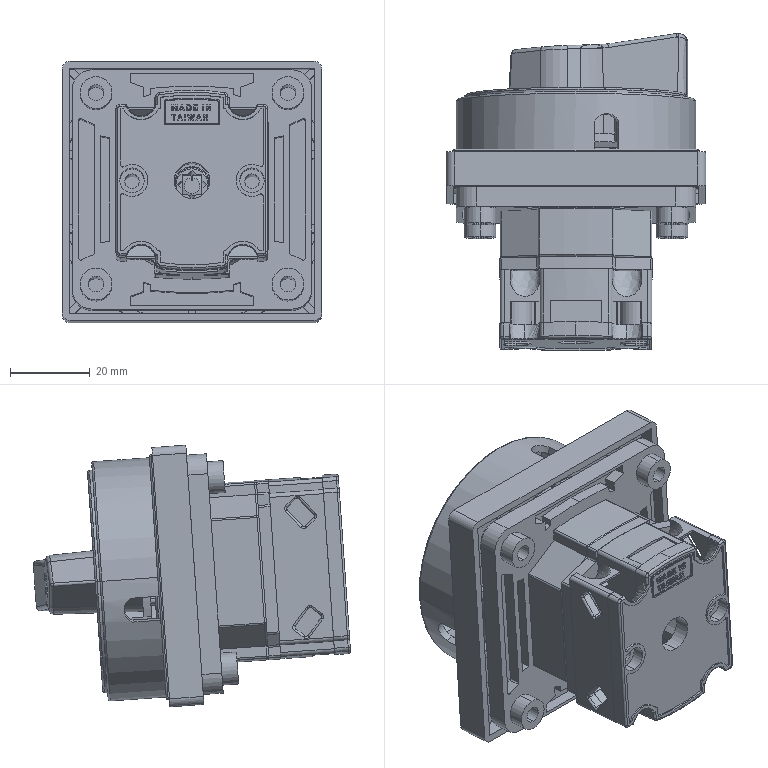Part | SolidWorks | features BaseBody 13 | 13 solids | 2462 faces | box 65 x 79.307 x 65.435 mm | volume 93271 mm3 | plane 1069 | cylinder 925 | torus 210 | spline 110 | sphere 76 | cone 72 | commonest cylinder face diameters 1 x196 0.4 x120 0.6 x104 10 x56 2 x49 6 x34